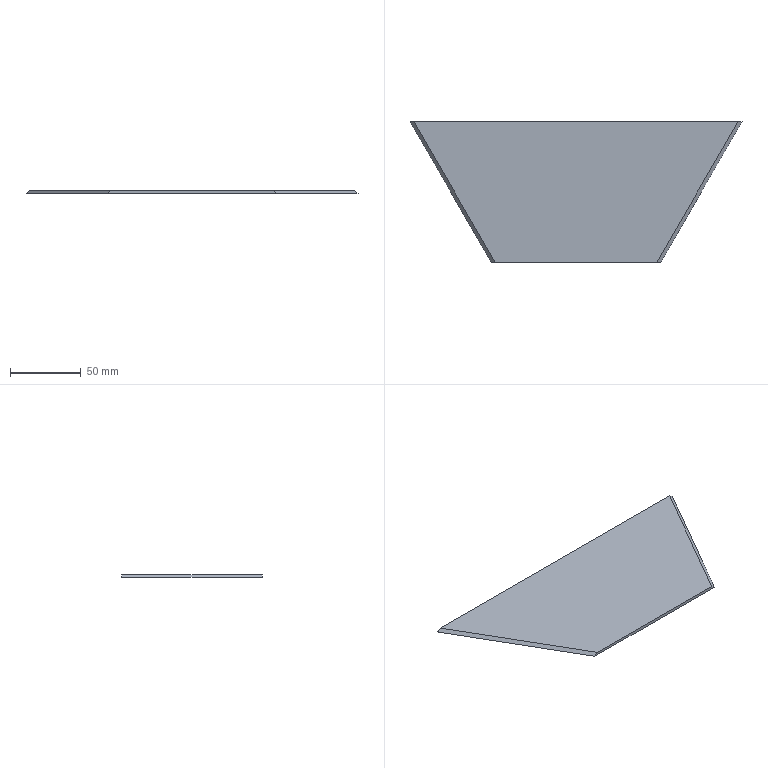Part | NX | 1 solid | 6 faces | box 235.47 x 100 x 2 mm | volume 34997 mm3 | plane 6
STEP:
#1=CARTESIAN_POINT('',(2.752,0.,2.));
#2=VERTEX_POINT('',#1);
#3=CARTESIAN_POINT('',(117.248,0.,2.));
#4=VERTEX_POINT('',#3);
#5=CARTESIAN_POINT('',(0.,0.,2.));
#6=DIRECTION('',(1.,0.,0.));
#7=VECTOR('',#6,1.);
#8=LINE('',#5,#7);
#9=EDGE_CURVE('',#2,#4,#8,.T.);
#10=ORIENTED_EDGE('',*,*,#9,.F.);
#11=CARTESIAN_POINT('',(0.,0.,0.));
#12=VERTEX_POINT('',#11);
#13=CARTESIAN_POINT('',(-35.481,0.,-25.783));
#14=DIRECTION('',(-0.809,0.,-0.5879));
#15=VECTOR('',#14,1.);
#16=LINE('',#13,#15);
#17=EDGE_CURVE('',#2,#12,#16,.T.);
#18=ORIENTED_EDGE('',*,*,#17,.T.);
#19=CARTESIAN_POINT('',(120.,0.,0.));
#20=VERTEX_POINT('',#19);
#21=CARTESIAN_POINT('',(0.,0.,0.));
#22=DIRECTION('',(1.,0.,0.));
#23=VECTOR('',#22,1.);
#24=LINE('',#21,#23);
#25=EDGE_CURVE('',#12,#20,#24,.T.);
#26=ORIENTED_EDGE('',*,*,#25,.T.);
#27=CARTESIAN_POINT('',(116.957,0.,2.211));
#28=DIRECTION('',(-0.809,0.,0.5879));
#29=VECTOR('',#28,1.);
#30=LINE('',#27,#29);
#31=EDGE_CURVE('',#20,#4,#30,.T.);
#32=ORIENTED_EDGE('',*,*,#31,.T.);
#33=EDGE_LOOP('',(#10,#18,#26,#32));
#34=FACE_OUTER_BOUND('',#33,.T.);
#35=CARTESIAN_POINT('',(0.,0.,2.));
#36=DIRECTION('',(0.,1.,0.));
#37=DIRECTION('',(0.,0.,1.));
#38=AXIS2_PLACEMENT_3D('',#35,#36,#37);
#39=PLANE('',#38);
#40=ADVANCED_FACE('',(#34),#39,.F.);
#41=CARTESIAN_POINT('',(177.735,100.,0.));
#42=VERTEX_POINT('',#41);
#43=CARTESIAN_POINT('',(-57.735,100.,0.));
#44=VERTEX_POINT('',#43);
#45=CARTESIAN_POINT('',(-57.735,100.,0.));
#46=DIRECTION('',(-1.,0.,0.));
#47=VECTOR('',#46,1.);
#48=LINE('',#45,#47);
#49=EDGE_CURVE('',#42,#44,#48,.T.);
#50=ORIENTED_EDGE('',*,*,#49,.T.);
#51=CARTESIAN_POINT('',(-54.983,100.,2.));
#52=VERTEX_POINT('',#51);
#53=CARTESIAN_POINT('',(-55.433,100.,1.673));
#54=DIRECTION('',(0.809,0.,0.5879));
#55=VECTOR('',#54,1.);
#56=LINE('',#53,#55);
#57=EDGE_CURVE('',#44,#52,#56,.T.);
#58=ORIENTED_EDGE('',*,*,#57,.T.);
#59=CARTESIAN_POINT('',(174.983,100.,2.));
#60=VERTEX_POINT('',#59);
#61=CARTESIAN_POINT('',(-57.735,100.,2.));
#62=DIRECTION('',(-1.,0.,0.));
#63=VECTOR('',#62,1.);
#64=LINE('',#61,#63);
#65=EDGE_CURVE('',#60,#52,#64,.T.);
#66=ORIENTED_EDGE('',*,*,#65,.F.);
#67=CARTESIAN_POINT('',(136.909,100.,29.668));
#68=DIRECTION('',(0.809,0.,-0.5879));
#69=VECTOR('',#68,1.);
#70=LINE('',#67,#69);
#71=EDGE_CURVE('',#60,#42,#70,.T.);
#72=ORIENTED_EDGE('',*,*,#71,.T.);
#73=EDGE_LOOP('',(#50,#58,#66,#72));
#74=FACE_OUTER_BOUND('',#73,.T.);
#75=CARTESIAN_POINT('',(-57.735,100.,2.));
#76=DIRECTION('',(0.,-1.,0.));
#77=DIRECTION('',(0.,0.,-1.));
#78=AXIS2_PLACEMENT_3D('',#75,#76,#77);
#79=PLANE('',#78);
#80=ADVANCED_FACE('',(#74),#79,.F.);
#81=ORIENTED_EDGE('',*,*,#65,.T.);
#82=CARTESIAN_POINT('',(-55.671,101.192,2.));
#83=DIRECTION('',(0.5,-0.866,0.));
#84=VECTOR('',#83,1.);
#85=LINE('',#82,#84);
#86=EDGE_CURVE('',#52,#2,#85,.T.);
#87=ORIENTED_EDGE('',*,*,#86,.T.);
#88=ORIENTED_EDGE('',*,*,#9,.T.);
#89=CARTESIAN_POINT('',(116.803,-0.7698,2.));
#90=DIRECTION('',(0.5,0.866,0.));
#91=VECTOR('',#90,1.);
#92=LINE('',#89,#91);
#93=EDGE_CURVE('',#4,#60,#92,.T.);
#94=ORIENTED_EDGE('',*,*,#93,.T.);
#95=EDGE_LOOP('',(#81,#87,#88,#94));
#96=FACE_OUTER_BOUND('',#95,.T.);
#97=CARTESIAN_POINT('',(-57.735,100.,2.));
#98=DIRECTION('',(0.,0.,-1.));
#99=DIRECTION('',(-1.,0.,0.));
#100=AXIS2_PLACEMENT_3D('',#97,#98,#99);
#101=PLANE('',#100);
#102=ADVANCED_FACE('',(#96),#101,.F.);
#103=CARTESIAN_POINT('',(0.,0.,0.));
#104=DIRECTION('',(0.5,-0.866,0.));
#105=VECTOR('',#104,1.);
#106=LINE('',#103,#105);
#107=EDGE_CURVE('',#44,#12,#106,.T.);
#108=ORIENTED_EDGE('',*,*,#107,.F.);
#109=ORIENTED_EDGE('',*,*,#49,.F.);
#110=CARTESIAN_POINT('',(120.,0.,0.));
#111=DIRECTION('',(0.5,0.866,0.));
#112=VECTOR('',#111,1.);
#113=LINE('',#110,#112);
#114=EDGE_CURVE('',#20,#42,#113,.T.);
#115=ORIENTED_EDGE('',*,*,#114,.F.);
#116=ORIENTED_EDGE('',*,*,#25,.F.);
#117=EDGE_LOOP('',(#108,#109,#115,#116));
#118=FACE_OUTER_BOUND('',#117,.T.);
#119=CARTESIAN_POINT('',(-57.735,100.,0.));
#120=DIRECTION('',(0.,0.,-1.));
#121=DIRECTION('',(-1.,0.,0.));
#122=AXIS2_PLACEMENT_3D('',#119,#120,#121);
#123=PLANE('',#122);
#124=ADVANCED_FACE('',(#118),#123,.T.);
#125=ORIENTED_EDGE('',*,*,#31,.F.);
#126=ORIENTED_EDGE('',*,*,#114,.T.);
#127=ORIENTED_EDGE('',*,*,#71,.F.);
#128=ORIENTED_EDGE('',*,*,#93,.F.);
#129=EDGE_LOOP('',(#125,#126,#127,#128));
#130=FACE_OUTER_BOUND('',#129,.T.);
#131=CARTESIAN_POINT('',(116.803,-0.7698,2.));
#132=DIRECTION('',(-0.5567,0.3214,-0.766));
#133=DIRECTION('',(-0.809,0.,0.5879));
#134=AXIS2_PLACEMENT_3D('',#131,#132,#133);
#135=PLANE('',#134);
#136=ADVANCED_FACE('',(#130),#135,.F.);
#137=ORIENTED_EDGE('',*,*,#57,.F.);
#138=ORIENTED_EDGE('',*,*,#107,.T.);
#139=ORIENTED_EDGE('',*,*,#17,.F.);
#140=ORIENTED_EDGE('',*,*,#86,.F.);
#141=EDGE_LOOP('',(#137,#138,#139,#140));
#142=FACE_OUTER_BOUND('',#141,.T.);
#143=CARTESIAN_POINT('',(-55.671,101.192,2.));
#144=DIRECTION('',(0.5567,0.3214,-0.766));
#145=DIRECTION('',(-0.809,0.,-0.5879));
#146=AXIS2_PLACEMENT_3D('',#143,#144,#145);
#147=PLANE('',#146);
#148=ADVANCED_FACE('',(#142),#147,.F.);
#149=CLOSED_SHELL('',(#40,#80,#102,#124,#136,#148));
#150=MANIFOLD_SOLID_BREP('',#149);
#151=(LENGTH_UNIT()NAMED_UNIT(*)SI_UNIT(.MILLI.,.METRE.));
#152=UNCERTAINTY_MEASURE_WITH_UNIT(LENGTH_MEASURE(0.00002),#151,'','');
#153=(NAMED_UNIT(*)PLANE_ANGLE_UNIT()SI_UNIT($,.RADIAN.));
#154=PLANE_ANGLE_MEASURE_WITH_UNIT(PLANE_ANGLE_MEASURE(0.01745),#153);
#155=DIMENSIONAL_EXPONENTS(0.,0.,0.,0.,0.,0.,0.);
#156=(CONVERSION_BASED_UNIT('DEGREE',#154)NAMED_UNIT(#155)PLANE_ANGLE_UNIT());
#157=(NAMED_UNIT(*)SI_UNIT($,.STERADIAN.)SOLID_ANGLE_UNIT());
#158=(GEOMETRIC_REPRESENTATION_CONTEXT(3)GLOBAL_UNCERTAINTY_ASSIGNED_CONTEXT((#152))GLOBAL_UNIT_ASSIGNED_CONTEXT((#151,#156,#157))REPRESENTATION_CONTEXT('',''));
#159=ADVANCED_BREP_SHAPE_REPRESENTATION('',(#150),#158);